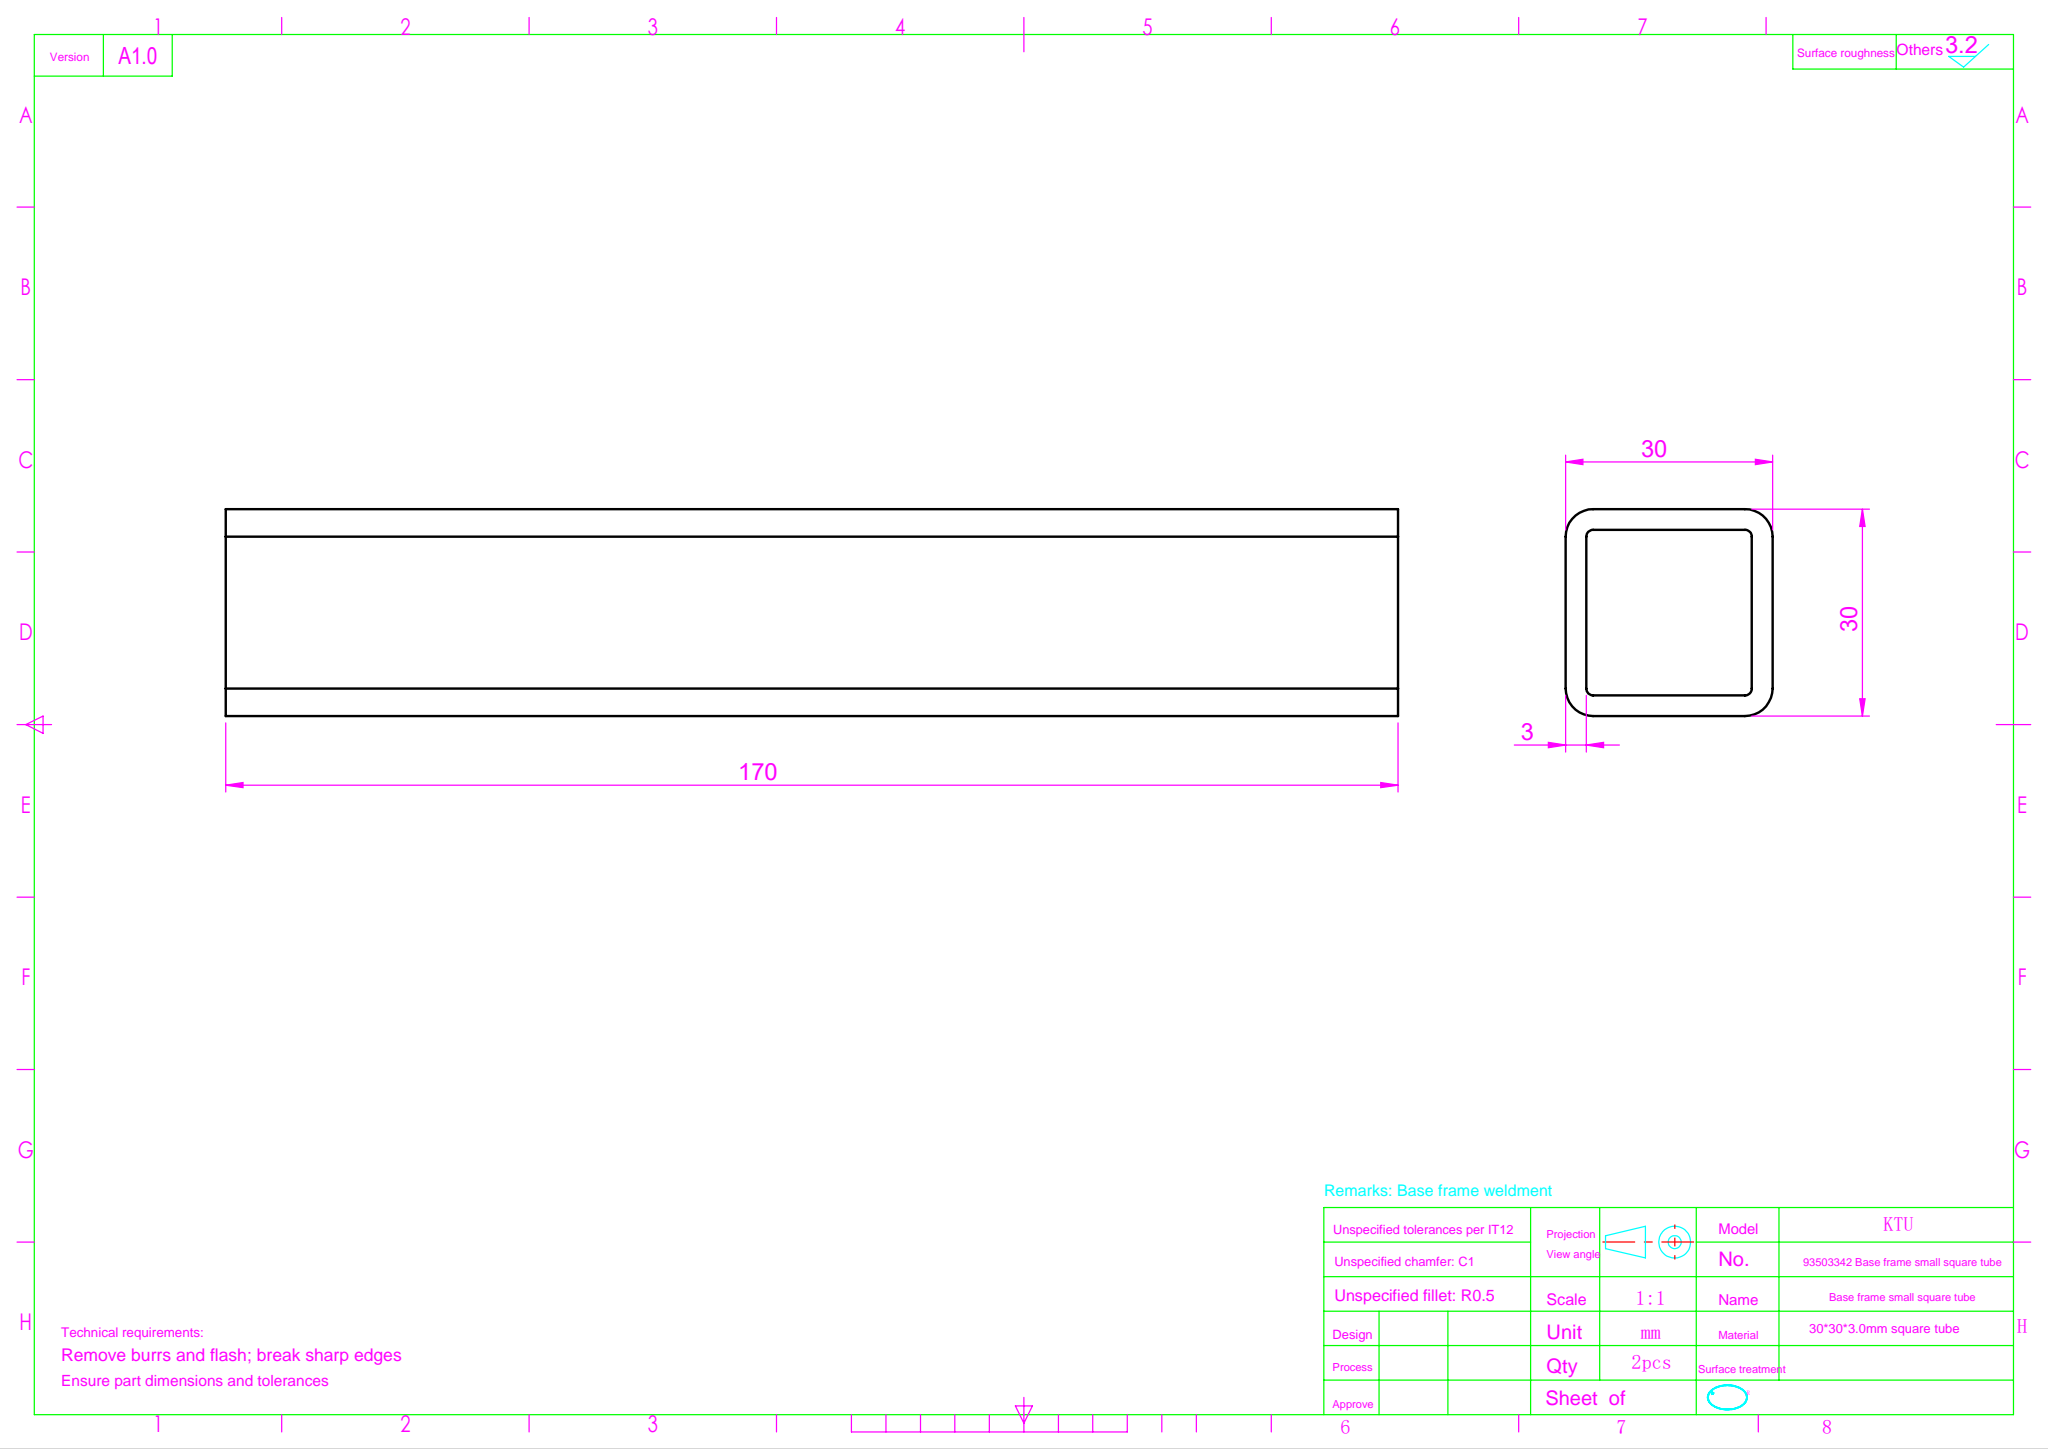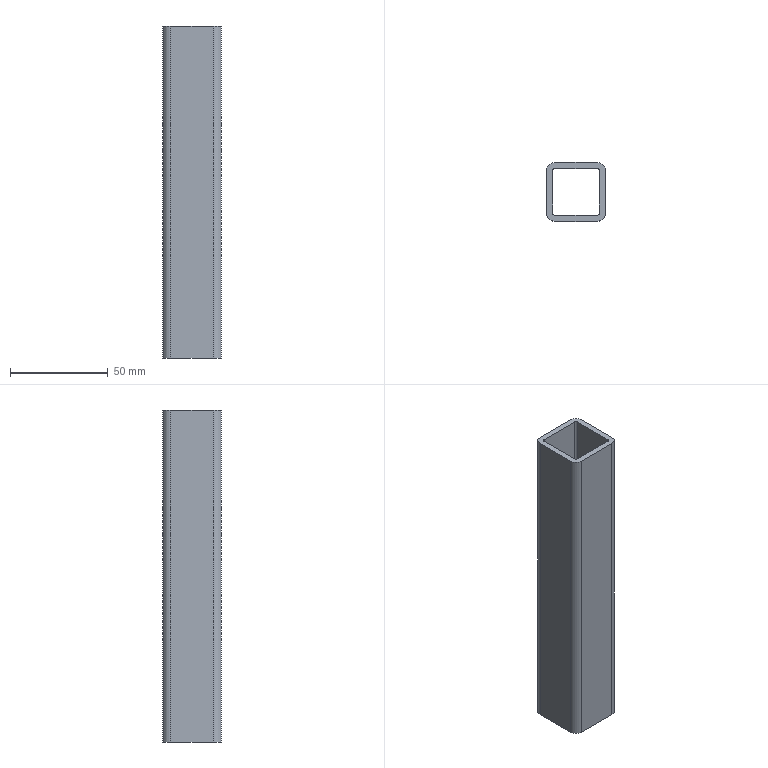Part | SolidWorks | features ExtruThin 1 | 1 solid | 18 faces | box 30 x 30 x 170 mm | volume 52891 mm3 | plane 10 | cylinder 8 | commonest cylinder face diameters 2 x4 8 x4
STEP:
#1=CARTESIAN_POINT('',(15.,11.,85.));
#2=VERTEX_POINT('',#1);
#3=CARTESIAN_POINT('',(11.,15.,85.));
#4=VERTEX_POINT('',#3);
#5=CARTESIAN_POINT('',(11.,11.,85.));
#6=DIRECTION('',(0.,0.,1.));
#7=DIRECTION('',(-1.,0.,0.));
#8=AXIS2_PLACEMENT_3D('',#5,#6,#7);
#9=CIRCLE('',#8,4.);
#10=EDGE_CURVE('',#2,#4,#9,.T.);
#11=ORIENTED_EDGE('',*,*,#10,.T.);
#12=CARTESIAN_POINT('',(-11.,15.,85.));
#13=VERTEX_POINT('',#12);
#14=CARTESIAN_POINT('',(-11.,15.,85.));
#15=DIRECTION('',(-1.,0.,0.));
#16=VECTOR('',#15,1000.);
#17=LINE('',#14,#16);
#18=EDGE_CURVE('',#4,#13,#17,.T.);
#19=ORIENTED_EDGE('',*,*,#18,.T.);
#20=CARTESIAN_POINT('',(-15.,11.,85.));
#21=VERTEX_POINT('',#20);
#22=CARTESIAN_POINT('',(-11.,11.,85.));
#23=DIRECTION('',(0.,0.,1.));
#24=DIRECTION('',(1.,0.,0.));
#25=AXIS2_PLACEMENT_3D('',#22,#23,#24);
#26=CIRCLE('',#25,4.);
#27=EDGE_CURVE('',#13,#21,#26,.T.);
#28=ORIENTED_EDGE('',*,*,#27,.T.);
#29=CARTESIAN_POINT('',(-15.,-11.,85.));
#30=VERTEX_POINT('',#29);
#31=CARTESIAN_POINT('',(-15.,11.,85.));
#32=DIRECTION('',(0.,-1.,0.));
#33=VECTOR('',#32,1000.);
#34=LINE('',#31,#33);
#35=EDGE_CURVE('',#21,#30,#34,.T.);
#36=ORIENTED_EDGE('',*,*,#35,.T.);
#37=CARTESIAN_POINT('',(-11.,-15.,85.));
#38=VERTEX_POINT('',#37);
#39=CARTESIAN_POINT('',(-11.,-11.,85.));
#40=DIRECTION('',(0.,0.,1.));
#41=DIRECTION('',(1.,0.,0.));
#42=AXIS2_PLACEMENT_3D('',#39,#40,#41);
#43=CIRCLE('',#42,4.);
#44=EDGE_CURVE('',#30,#38,#43,.T.);
#45=ORIENTED_EDGE('',*,*,#44,.T.);
#46=CARTESIAN_POINT('',(11.,-15.,85.));
#47=VERTEX_POINT('',#46);
#48=CARTESIAN_POINT('',(-11.,-15.,85.));
#49=DIRECTION('',(1.,0.,0.));
#50=VECTOR('',#49,1000.);
#51=LINE('',#48,#50);
#52=EDGE_CURVE('',#38,#47,#51,.T.);
#53=ORIENTED_EDGE('',*,*,#52,.T.);
#54=CARTESIAN_POINT('',(15.,-11.,85.));
#55=VERTEX_POINT('',#54);
#56=CARTESIAN_POINT('',(11.,-11.,85.));
#57=DIRECTION('',(0.,0.,1.));
#58=DIRECTION('',(1.,0.,0.));
#59=AXIS2_PLACEMENT_3D('',#56,#57,#58);
#60=CIRCLE('',#59,4.);
#61=EDGE_CURVE('',#47,#55,#60,.T.);
#62=ORIENTED_EDGE('',*,*,#61,.T.);
#63=CARTESIAN_POINT('',(15.,11.,85.));
#64=DIRECTION('',(0.,1.,0.));
#65=VECTOR('',#64,1000.);
#66=LINE('',#63,#65);
#67=EDGE_CURVE('',#55,#2,#66,.T.);
#68=ORIENTED_EDGE('',*,*,#67,.T.);
#69=EDGE_LOOP('',(#11,#19,#28,#36,#45,#53,#62,#68));
#70=FACE_OUTER_BOUND('',#69,.T.);
#71=CARTESIAN_POINT('',(11.,12.,85.));
#72=VERTEX_POINT('',#71);
#73=CARTESIAN_POINT('',(-11.,12.,85.));
#74=VERTEX_POINT('',#73);
#75=CARTESIAN_POINT('',(11.,12.,85.));
#76=DIRECTION('',(-1.,0.,0.));
#77=VECTOR('',#76,1000.);
#78=LINE('',#75,#77);
#79=EDGE_CURVE('',#72,#74,#78,.T.);
#80=ORIENTED_EDGE('',*,*,#79,.F.);
#81=CARTESIAN_POINT('',(12.,11.,85.));
#82=VERTEX_POINT('',#81);
#83=CARTESIAN_POINT('',(11.,11.,85.));
#84=DIRECTION('',(0.,0.,1.));
#85=DIRECTION('',(-1.,0.,0.));
#86=AXIS2_PLACEMENT_3D('',#83,#84,#85);
#87=CIRCLE('',#86,1.);
#88=EDGE_CURVE('',#82,#72,#87,.T.);
#89=ORIENTED_EDGE('',*,*,#88,.F.);
#90=CARTESIAN_POINT('',(12.,-11.,85.));
#91=VERTEX_POINT('',#90);
#92=CARTESIAN_POINT('',(12.,11.,85.));
#93=DIRECTION('',(0.,1.,0.));
#94=VECTOR('',#93,1000.);
#95=LINE('',#92,#94);
#96=EDGE_CURVE('',#91,#82,#95,.T.);
#97=ORIENTED_EDGE('',*,*,#96,.F.);
#98=CARTESIAN_POINT('',(11.,-12.,85.));
#99=VERTEX_POINT('',#98);
#100=CARTESIAN_POINT('',(11.,-11.,85.));
#101=DIRECTION('',(0.,0.,1.));
#102=DIRECTION('',(-1.,0.,0.));
#103=AXIS2_PLACEMENT_3D('',#100,#101,#102);
#104=CIRCLE('',#103,1.);
#105=EDGE_CURVE('',#99,#91,#104,.T.);
#106=ORIENTED_EDGE('',*,*,#105,.F.);
#107=CARTESIAN_POINT('',(-11.,-12.,85.));
#108=VERTEX_POINT('',#107);
#109=CARTESIAN_POINT('',(11.,-12.,85.));
#110=DIRECTION('',(1.,0.,0.));
#111=VECTOR('',#110,1000.);
#112=LINE('',#109,#111);
#113=EDGE_CURVE('',#108,#99,#112,.T.);
#114=ORIENTED_EDGE('',*,*,#113,.F.);
#115=CARTESIAN_POINT('',(-12.,-11.,85.));
#116=VERTEX_POINT('',#115);
#117=CARTESIAN_POINT('',(-11.,-11.,85.));
#118=DIRECTION('',(0.,0.,1.));
#119=DIRECTION('',(-1.,0.,0.));
#120=AXIS2_PLACEMENT_3D('',#117,#118,#119);
#121=CIRCLE('',#120,1.);
#122=EDGE_CURVE('',#116,#108,#121,.T.);
#123=ORIENTED_EDGE('',*,*,#122,.F.);
#124=CARTESIAN_POINT('',(-12.,11.,85.));
#125=VERTEX_POINT('',#124);
#126=CARTESIAN_POINT('',(-12.,11.,85.));
#127=DIRECTION('',(0.,-1.,0.));
#128=VECTOR('',#127,1000.);
#129=LINE('',#126,#128);
#130=EDGE_CURVE('',#125,#116,#129,.T.);
#131=ORIENTED_EDGE('',*,*,#130,.F.);
#132=CARTESIAN_POINT('',(-11.,11.,85.));
#133=DIRECTION('',(0.,0.,1.));
#134=DIRECTION('',(-1.,0.,0.));
#135=AXIS2_PLACEMENT_3D('',#132,#133,#134);
#136=CIRCLE('',#135,1.);
#137=EDGE_CURVE('',#74,#125,#136,.T.);
#138=ORIENTED_EDGE('',*,*,#137,.F.);
#139=EDGE_LOOP('',(#80,#89,#97,#106,#114,#123,#131,#138));
#140=FACE_BOUND('',#139,.T.);
#141=CARTESIAN_POINT('',(11.,11.,85.));
#142=DIRECTION('',(0.,0.,1.));
#143=DIRECTION('',(1.,0.,0.));
#144=AXIS2_PLACEMENT_3D('',#141,#142,#143);
#145=PLANE('',#144);
#146=ADVANCED_FACE('',(#70,#140),#145,.T.);
#147=CARTESIAN_POINT('',(15.,11.,-85.));
#148=VERTEX_POINT('',#147);
#149=CARTESIAN_POINT('',(11.,15.,-85.));
#150=VERTEX_POINT('',#149);
#151=CARTESIAN_POINT('',(11.,11.,-85.));
#152=DIRECTION('',(0.,0.,1.));
#153=DIRECTION('',(-1.,0.,0.));
#154=AXIS2_PLACEMENT_3D('',#151,#152,#153);
#155=CIRCLE('',#154,4.);
#156=EDGE_CURVE('',#148,#150,#155,.T.);
#157=ORIENTED_EDGE('',*,*,#156,.F.);
#158=CARTESIAN_POINT('',(15.,-11.,-85.));
#159=VERTEX_POINT('',#158);
#160=CARTESIAN_POINT('',(15.,11.,-85.));
#161=DIRECTION('',(0.,1.,0.));
#162=VECTOR('',#161,1000.);
#163=LINE('',#160,#162);
#164=EDGE_CURVE('',#159,#148,#163,.T.);
#165=ORIENTED_EDGE('',*,*,#164,.F.);
#166=CARTESIAN_POINT('',(11.,-15.,-85.));
#167=VERTEX_POINT('',#166);
#168=CARTESIAN_POINT('',(11.,-11.,-85.));
#169=DIRECTION('',(0.,0.,1.));
#170=DIRECTION('',(1.,0.,0.));
#171=AXIS2_PLACEMENT_3D('',#168,#169,#170);
#172=CIRCLE('',#171,4.);
#173=EDGE_CURVE('',#167,#159,#172,.T.);
#174=ORIENTED_EDGE('',*,*,#173,.F.);
#175=CARTESIAN_POINT('',(-11.,-15.,-85.));
#176=VERTEX_POINT('',#175);
#177=CARTESIAN_POINT('',(-11.,-15.,-85.));
#178=DIRECTION('',(1.,0.,0.));
#179=VECTOR('',#178,1000.);
#180=LINE('',#177,#179);
#181=EDGE_CURVE('',#176,#167,#180,.T.);
#182=ORIENTED_EDGE('',*,*,#181,.F.);
#183=CARTESIAN_POINT('',(-15.,-11.,-85.));
#184=VERTEX_POINT('',#183);
#185=CARTESIAN_POINT('',(-11.,-11.,-85.));
#186=DIRECTION('',(0.,0.,1.));
#187=DIRECTION('',(1.,0.,0.));
#188=AXIS2_PLACEMENT_3D('',#185,#186,#187);
#189=CIRCLE('',#188,4.);
#190=EDGE_CURVE('',#184,#176,#189,.T.);
#191=ORIENTED_EDGE('',*,*,#190,.F.);
#192=CARTESIAN_POINT('',(-15.,11.,-85.));
#193=VERTEX_POINT('',#192);
#194=CARTESIAN_POINT('',(-15.,11.,-85.));
#195=DIRECTION('',(0.,-1.,0.));
#196=VECTOR('',#195,1000.);
#197=LINE('',#194,#196);
#198=EDGE_CURVE('',#193,#184,#197,.T.);
#199=ORIENTED_EDGE('',*,*,#198,.F.);
#200=CARTESIAN_POINT('',(-11.,15.,-85.));
#201=VERTEX_POINT('',#200);
#202=CARTESIAN_POINT('',(-11.,11.,-85.));
#203=DIRECTION('',(0.,0.,1.));
#204=DIRECTION('',(1.,0.,0.));
#205=AXIS2_PLACEMENT_3D('',#202,#203,#204);
#206=CIRCLE('',#205,4.);
#207=EDGE_CURVE('',#201,#193,#206,.T.);
#208=ORIENTED_EDGE('',*,*,#207,.F.);
#209=CARTESIAN_POINT('',(-11.,15.,-85.));
#210=DIRECTION('',(-1.,0.,0.));
#211=VECTOR('',#210,1000.);
#212=LINE('',#209,#211);
#213=EDGE_CURVE('',#150,#201,#212,.T.);
#214=ORIENTED_EDGE('',*,*,#213,.F.);
#215=EDGE_LOOP('',(#157,#165,#174,#182,#191,#199,#208,#214));
#216=FACE_OUTER_BOUND('',#215,.T.);
#217=CARTESIAN_POINT('',(12.,11.,-85.));
#218=VERTEX_POINT('',#217);
#219=CARTESIAN_POINT('',(11.,12.,-85.));
#220=VERTEX_POINT('',#219);
#221=CARTESIAN_POINT('',(11.,11.,-85.));
#222=DIRECTION('',(0.,0.,1.));
#223=DIRECTION('',(-1.,0.,0.));
#224=AXIS2_PLACEMENT_3D('',#221,#222,#223);
#225=CIRCLE('',#224,1.);
#226=EDGE_CURVE('',#218,#220,#225,.T.);
#227=ORIENTED_EDGE('',*,*,#226,.T.);
#228=CARTESIAN_POINT('',(-11.,12.,-85.));
#229=VERTEX_POINT('',#228);
#230=CARTESIAN_POINT('',(11.,12.,-85.));
#231=DIRECTION('',(-1.,0.,0.));
#232=VECTOR('',#231,1000.);
#233=LINE('',#230,#232);
#234=EDGE_CURVE('',#220,#229,#233,.T.);
#235=ORIENTED_EDGE('',*,*,#234,.T.);
#236=CARTESIAN_POINT('',(-12.,11.,-85.));
#237=VERTEX_POINT('',#236);
#238=CARTESIAN_POINT('',(-11.,11.,-85.));
#239=DIRECTION('',(0.,0.,1.));
#240=DIRECTION('',(-1.,0.,0.));
#241=AXIS2_PLACEMENT_3D('',#238,#239,#240);
#242=CIRCLE('',#241,1.);
#243=EDGE_CURVE('',#229,#237,#242,.T.);
#244=ORIENTED_EDGE('',*,*,#243,.T.);
#245=CARTESIAN_POINT('',(-12.,-11.,-85.));
#246=VERTEX_POINT('',#245);
#247=CARTESIAN_POINT('',(-12.,11.,-85.));
#248=DIRECTION('',(0.,-1.,0.));
#249=VECTOR('',#248,1000.);
#250=LINE('',#247,#249);
#251=EDGE_CURVE('',#237,#246,#250,.T.);
#252=ORIENTED_EDGE('',*,*,#251,.T.);
#253=CARTESIAN_POINT('',(-11.,-12.,-85.));
#254=VERTEX_POINT('',#253);
#255=CARTESIAN_POINT('',(-11.,-11.,-85.));
#256=DIRECTION('',(0.,0.,1.));
#257=DIRECTION('',(-1.,0.,0.));
#258=AXIS2_PLACEMENT_3D('',#255,#256,#257);
#259=CIRCLE('',#258,1.);
#260=EDGE_CURVE('',#246,#254,#259,.T.);
#261=ORIENTED_EDGE('',*,*,#260,.T.);
#262=CARTESIAN_POINT('',(11.,-12.,-85.));
#263=VERTEX_POINT('',#262);
#264=CARTESIAN_POINT('',(11.,-12.,-85.));
#265=DIRECTION('',(1.,0.,0.));
#266=VECTOR('',#265,1000.);
#267=LINE('',#264,#266);
#268=EDGE_CURVE('',#254,#263,#267,.T.);
#269=ORIENTED_EDGE('',*,*,#268,.T.);
#270=CARTESIAN_POINT('',(12.,-11.,-85.));
#271=VERTEX_POINT('',#270);
#272=CARTESIAN_POINT('',(11.,-11.,-85.));
#273=DIRECTION('',(0.,0.,1.));
#274=DIRECTION('',(-1.,0.,0.));
#275=AXIS2_PLACEMENT_3D('',#272,#273,#274);
#276=CIRCLE('',#275,1.);
#277=EDGE_CURVE('',#263,#271,#276,.T.);
#278=ORIENTED_EDGE('',*,*,#277,.T.);
#279=CARTESIAN_POINT('',(12.,11.,-85.));
#280=DIRECTION('',(0.,1.,0.));
#281=VECTOR('',#280,1000.);
#282=LINE('',#279,#281);
#283=EDGE_CURVE('',#271,#218,#282,.T.);
#284=ORIENTED_EDGE('',*,*,#283,.T.);
#285=EDGE_LOOP('',(#227,#235,#244,#252,#261,#269,#278,#284));
#286=FACE_BOUND('',#285,.T.);
#287=CARTESIAN_POINT('',(11.,11.,-85.));
#288=DIRECTION('',(0.,0.,1.));
#289=DIRECTION('',(1.,0.,0.));
#290=AXIS2_PLACEMENT_3D('',#287,#288,#289);
#291=PLANE('',#290);
#292=ADVANCED_FACE('',(#216,#286),#291,.F.);
#293=ORIENTED_EDGE('',*,*,#156,.T.);
#294=CARTESIAN_POINT('',(11.,15.,85.));
#295=DIRECTION('',(0.,0.,-1.));
#296=VECTOR('',#295,1000.);
#297=LINE('',#294,#296);
#298=EDGE_CURVE('',#4,#150,#297,.T.);
#299=ORIENTED_EDGE('',*,*,#298,.F.);
#300=ORIENTED_EDGE('',*,*,#10,.F.);
#301=CARTESIAN_POINT('',(15.,11.,85.));
#302=DIRECTION('',(0.,0.,-1.));
#303=VECTOR('',#302,1000.);
#304=LINE('',#301,#303);
#305=EDGE_CURVE('',#2,#148,#304,.T.);
#306=ORIENTED_EDGE('',*,*,#305,.T.);
#307=EDGE_LOOP('',(#293,#299,#300,#306));
#308=FACE_OUTER_BOUND('',#307,.T.);
#309=CARTESIAN_POINT('',(11.,11.,85.));
#310=DIRECTION('',(0.,0.,-1.));
#311=DIRECTION('',(-1.,0.,0.));
#312=AXIS2_PLACEMENT_3D('',#309,#310,#311);
#313=CYLINDRICAL_SURFACE('',#312,4.);
#314=ADVANCED_FACE('',(#308),#313,.T.);
#315=ORIENTED_EDGE('',*,*,#213,.T.);
#316=CARTESIAN_POINT('',(-11.,15.,85.));
#317=DIRECTION('',(0.,0.,-1.));
#318=VECTOR('',#317,1000.);
#319=LINE('',#316,#318);
#320=EDGE_CURVE('',#13,#201,#319,.T.);
#321=ORIENTED_EDGE('',*,*,#320,.F.);
#322=ORIENTED_EDGE('',*,*,#18,.F.);
#323=ORIENTED_EDGE('',*,*,#298,.T.);
#324=EDGE_LOOP('',(#315,#321,#322,#323));
#325=FACE_OUTER_BOUND('',#324,.T.);
#326=CARTESIAN_POINT('',(-11.,15.,85.));
#327=DIRECTION('',(0.,-1.,0.));
#328=DIRECTION('',(0.,0.,-1.));
#329=AXIS2_PLACEMENT_3D('',#326,#327,#328);
#330=PLANE('',#329);
#331=ADVANCED_FACE('',(#325),#330,.F.);
#332=ORIENTED_EDGE('',*,*,#207,.T.);
#333=CARTESIAN_POINT('',(-15.,11.,85.));
#334=DIRECTION('',(0.,0.,-1.));
#335=VECTOR('',#334,1000.);
#336=LINE('',#333,#335);
#337=EDGE_CURVE('',#21,#193,#336,.T.);
#338=ORIENTED_EDGE('',*,*,#337,.F.);
#339=ORIENTED_EDGE('',*,*,#27,.F.);
#340=ORIENTED_EDGE('',*,*,#320,.T.);
#341=EDGE_LOOP('',(#332,#338,#339,#340));
#342=FACE_OUTER_BOUND('',#341,.T.);
#343=CARTESIAN_POINT('',(-11.,11.,85.));
#344=DIRECTION('',(0.,0.,-1.));
#345=DIRECTION('',(-1.,0.,0.));
#346=AXIS2_PLACEMENT_3D('',#343,#344,#345);
#347=CYLINDRICAL_SURFACE('',#346,4.);
#348=ADVANCED_FACE('',(#342),#347,.T.);
#349=ORIENTED_EDGE('',*,*,#198,.T.);
#350=CARTESIAN_POINT('',(-15.,-11.,85.));
#351=DIRECTION('',(0.,0.,-1.));
#352=VECTOR('',#351,1000.);
#353=LINE('',#350,#352);
#354=EDGE_CURVE('',#30,#184,#353,.T.);
#355=ORIENTED_EDGE('',*,*,#354,.F.);
#356=ORIENTED_EDGE('',*,*,#35,.F.);
#357=ORIENTED_EDGE('',*,*,#337,.T.);
#358=EDGE_LOOP('',(#349,#355,#356,#357));
#359=FACE_OUTER_BOUND('',#358,.T.);
#360=CARTESIAN_POINT('',(-15.,11.,85.));
#361=DIRECTION('',(1.,0.,0.));
#362=DIRECTION('',(0.,1.,0.));
#363=AXIS2_PLACEMENT_3D('',#360,#361,#362);
#364=PLANE('',#363);
#365=ADVANCED_FACE('',(#359),#364,.F.);
#366=ORIENTED_EDGE('',*,*,#190,.T.);
#367=CARTESIAN_POINT('',(-11.,-15.,85.));
#368=DIRECTION('',(0.,0.,-1.));
#369=VECTOR('',#368,1000.);
#370=LINE('',#367,#369);
#371=EDGE_CURVE('',#38,#176,#370,.T.);
#372=ORIENTED_EDGE('',*,*,#371,.F.);
#373=ORIENTED_EDGE('',*,*,#44,.F.);
#374=ORIENTED_EDGE('',*,*,#354,.T.);
#375=EDGE_LOOP('',(#366,#372,#373,#374));
#376=FACE_OUTER_BOUND('',#375,.T.);
#377=CARTESIAN_POINT('',(-11.,-11.,85.));
#378=DIRECTION('',(0.,0.,-1.));
#379=DIRECTION('',(-1.,0.,0.));
#380=AXIS2_PLACEMENT_3D('',#377,#378,#379);
#381=CYLINDRICAL_SURFACE('',#380,4.);
#382=ADVANCED_FACE('',(#376),#381,.T.);
#383=ORIENTED_EDGE('',*,*,#181,.T.);
#384=CARTESIAN_POINT('',(11.,-15.,85.));
#385=DIRECTION('',(0.,0.,-1.));
#386=VECTOR('',#385,1000.);
#387=LINE('',#384,#386);
#388=EDGE_CURVE('',#47,#167,#387,.T.);
#389=ORIENTED_EDGE('',*,*,#388,.F.);
#390=ORIENTED_EDGE('',*,*,#52,.F.);
#391=ORIENTED_EDGE('',*,*,#371,.T.);
#392=EDGE_LOOP('',(#383,#389,#390,#391));
#393=FACE_OUTER_BOUND('',#392,.T.);
#394=CARTESIAN_POINT('',(-11.,-15.,85.));
#395=DIRECTION('',(0.,1.,0.));
#396=DIRECTION('',(0.,0.,1.));
#397=AXIS2_PLACEMENT_3D('',#394,#395,#396);
#398=PLANE('',#397);
#399=ADVANCED_FACE('',(#393),#398,.F.);
#400=ORIENTED_EDGE('',*,*,#173,.T.);
#401=CARTESIAN_POINT('',(15.,-11.,85.));
#402=DIRECTION('',(0.,0.,-1.));
#403=VECTOR('',#402,1000.);
#404=LINE('',#401,#403);
#405=EDGE_CURVE('',#55,#159,#404,.T.);
#406=ORIENTED_EDGE('',*,*,#405,.F.);
#407=ORIENTED_EDGE('',*,*,#61,.F.);
#408=ORIENTED_EDGE('',*,*,#388,.T.);
#409=EDGE_LOOP('',(#400,#406,#407,#408));
#410=FACE_OUTER_BOUND('',#409,.T.);
#411=CARTESIAN_POINT('',(11.,-11.,85.));
#412=DIRECTION('',(0.,0.,-1.));
#413=DIRECTION('',(-1.,0.,0.));
#414=AXIS2_PLACEMENT_3D('',#411,#412,#413);
#415=CYLINDRICAL_SURFACE('',#414,4.);
#416=ADVANCED_FACE('',(#410),#415,.T.);
#417=ORIENTED_EDGE('',*,*,#164,.T.);
#418=ORIENTED_EDGE('',*,*,#305,.F.);
#419=ORIENTED_EDGE('',*,*,#67,.F.);
#420=ORIENTED_EDGE('',*,*,#405,.T.);
#421=EDGE_LOOP('',(#417,#418,#419,#420));
#422=FACE_OUTER_BOUND('',#421,.T.);
#423=CARTESIAN_POINT('',(15.,11.,85.));
#424=DIRECTION('',(-1.,0.,0.));
#425=DIRECTION('',(0.,-1.,0.));
#426=AXIS2_PLACEMENT_3D('',#423,#424,#425);
#427=PLANE('',#426);
#428=ADVANCED_FACE('',(#422),#427,.F.);
#429=ORIENTED_EDGE('',*,*,#226,.F.);
#430=CARTESIAN_POINT('',(12.,11.,85.));
#431=DIRECTION('',(0.,0.,-1.));
#432=VECTOR('',#431,1000.);
#433=LINE('',#430,#432);
#434=EDGE_CURVE('',#82,#218,#433,.T.);
#435=ORIENTED_EDGE('',*,*,#434,.F.);
#436=ORIENTED_EDGE('',*,*,#88,.T.);
#437=CARTESIAN_POINT('',(11.,12.,85.));
#438=DIRECTION('',(0.,0.,-1.));
#439=VECTOR('',#438,1000.);
#440=LINE('',#437,#439);
#441=EDGE_CURVE('',#72,#220,#440,.T.);
#442=ORIENTED_EDGE('',*,*,#441,.T.);
#443=EDGE_LOOP('',(#429,#435,#436,#442));
#444=FACE_OUTER_BOUND('',#443,.T.);
#445=CARTESIAN_POINT('',(11.,11.,85.));
#446=DIRECTION('',(0.,0.,-1.));
#447=DIRECTION('',(-1.,0.,0.));
#448=AXIS2_PLACEMENT_3D('',#445,#446,#447);
#449=CYLINDRICAL_SURFACE('',#448,1.);
#450=ADVANCED_FACE('',(#444),#449,.F.);
#451=ORIENTED_EDGE('',*,*,#234,.F.);
#452=ORIENTED_EDGE('',*,*,#441,.F.);
#453=ORIENTED_EDGE('',*,*,#79,.T.);
#454=CARTESIAN_POINT('',(-11.,12.,85.));
#455=DIRECTION('',(0.,0.,-1.));
#456=VECTOR('',#455,1000.);
#457=LINE('',#454,#456);
#458=EDGE_CURVE('',#74,#229,#457,.T.);
#459=ORIENTED_EDGE('',*,*,#458,.T.);
#460=EDGE_LOOP('',(#451,#452,#453,#459));
#461=FACE_OUTER_BOUND('',#460,.T.);
#462=CARTESIAN_POINT('',(11.,12.,85.));
#463=DIRECTION('',(0.,-1.,0.));
#464=DIRECTION('',(0.,0.,-1.));
#465=AXIS2_PLACEMENT_3D('',#462,#463,#464);
#466=PLANE('',#465);
#467=ADVANCED_FACE('',(#461),#466,.T.);
#468=ORIENTED_EDGE('',*,*,#243,.F.);
#469=ORIENTED_EDGE('',*,*,#458,.F.);
#470=ORIENTED_EDGE('',*,*,#137,.T.);
#471=CARTESIAN_POINT('',(-12.,11.,85.));
#472=DIRECTION('',(0.,0.,-1.));
#473=VECTOR('',#472,1000.);
#474=LINE('',#471,#473);
#475=EDGE_CURVE('',#125,#237,#474,.T.);
#476=ORIENTED_EDGE('',*,*,#475,.T.);
#477=EDGE_LOOP('',(#468,#469,#470,#476));
#478=FACE_OUTER_BOUND('',#477,.T.);
#479=CARTESIAN_POINT('',(-11.,11.,85.));
#480=DIRECTION('',(0.,0.,-1.));
#481=DIRECTION('',(-1.,0.,0.));
#482=AXIS2_PLACEMENT_3D('',#479,#480,#481);
#483=CYLINDRICAL_SURFACE('',#482,1.);
#484=ADVANCED_FACE('',(#478),#483,.F.);
#485=ORIENTED_EDGE('',*,*,#251,.F.);
#486=ORIENTED_EDGE('',*,*,#475,.F.);
#487=ORIENTED_EDGE('',*,*,#130,.T.);
#488=CARTESIAN_POINT('',(-12.,-11.,85.));
#489=DIRECTION('',(0.,0.,-1.));
#490=VECTOR('',#489,1000.);
#491=LINE('',#488,#490);
#492=EDGE_CURVE('',#116,#246,#491,.T.);
#493=ORIENTED_EDGE('',*,*,#492,.T.);
#494=EDGE_LOOP('',(#485,#486,#487,#493));
#495=FACE_OUTER_BOUND('',#494,.T.);
#496=CARTESIAN_POINT('',(-12.,11.,85.));
#497=DIRECTION('',(1.,0.,0.));
#498=DIRECTION('',(0.,1.,0.));
#499=AXIS2_PLACEMENT_3D('',#496,#497,#498);
#500=PLANE('',#499);
#501=ADVANCED_FACE('',(#495),#500,.T.);
#502=ORIENTED_EDGE('',*,*,#260,.F.);
#503=ORIENTED_EDGE('',*,*,#492,.F.);
#504=ORIENTED_EDGE('',*,*,#122,.T.);
#505=CARTESIAN_POINT('',(-11.,-12.,85.));
#506=DIRECTION('',(0.,0.,-1.));
#507=VECTOR('',#506,1000.);
#508=LINE('',#505,#507);
#509=EDGE_CURVE('',#108,#254,#508,.T.);
#510=ORIENTED_EDGE('',*,*,#509,.T.);
#511=EDGE_LOOP('',(#502,#503,#504,#510));
#512=FACE_OUTER_BOUND('',#511,.T.);
#513=CARTESIAN_POINT('',(-11.,-11.,85.));
#514=DIRECTION('',(0.,0.,-1.));
#515=DIRECTION('',(-1.,0.,0.));
#516=AXIS2_PLACEMENT_3D('',#513,#514,#515);
#517=CYLINDRICAL_SURFACE('',#516,1.);
#518=ADVANCED_FACE('',(#512),#517,.F.);
#519=ORIENTED_EDGE('',*,*,#268,.F.);
#520=ORIENTED_EDGE('',*,*,#509,.F.);
#521=ORIENTED_EDGE('',*,*,#113,.T.);
#522=CARTESIAN_POINT('',(11.,-12.,85.));
#523=DIRECTION('',(0.,0.,-1.));
#524=VECTOR('',#523,1000.);
#525=LINE('',#522,#524);
#526=EDGE_CURVE('',#99,#263,#525,.T.);
#527=ORIENTED_EDGE('',*,*,#526,.T.);
#528=EDGE_LOOP('',(#519,#520,#521,#527));
#529=FACE_OUTER_BOUND('',#528,.T.);
#530=CARTESIAN_POINT('',(11.,-12.,85.));
#531=DIRECTION('',(0.,1.,0.));
#532=DIRECTION('',(0.,0.,1.));
#533=AXIS2_PLACEMENT_3D('',#530,#531,#532);
#534=PLANE('',#533);
#535=ADVANCED_FACE('',(#529),#534,.T.);
#536=ORIENTED_EDGE('',*,*,#277,.F.);
#537=ORIENTED_EDGE('',*,*,#526,.F.);
#538=ORIENTED_EDGE('',*,*,#105,.T.);
#539=CARTESIAN_POINT('',(12.,-11.,85.));
#540=DIRECTION('',(0.,0.,-1.));
#541=VECTOR('',#540,1000.);
#542=LINE('',#539,#541);
#543=EDGE_CURVE('',#91,#271,#542,.T.);
#544=ORIENTED_EDGE('',*,*,#543,.T.);
#545=EDGE_LOOP('',(#536,#537,#538,#544));
#546=FACE_OUTER_BOUND('',#545,.T.);
#547=CARTESIAN_POINT('',(11.,-11.,85.));
#548=DIRECTION('',(0.,0.,-1.));
#549=DIRECTION('',(-1.,0.,0.));
#550=AXIS2_PLACEMENT_3D('',#547,#548,#549);
#551=CYLINDRICAL_SURFACE('',#550,1.);
#552=ADVANCED_FACE('',(#546),#551,.F.);
#553=ORIENTED_EDGE('',*,*,#283,.F.);
#554=ORIENTED_EDGE('',*,*,#543,.F.);
#555=ORIENTED_EDGE('',*,*,#96,.T.);
#556=ORIENTED_EDGE('',*,*,#434,.T.);
#557=EDGE_LOOP('',(#553,#554,#555,#556));
#558=FACE_OUTER_BOUND('',#557,.T.);
#559=CARTESIAN_POINT('',(12.,11.,85.));
#560=DIRECTION('',(-1.,0.,0.));
#561=DIRECTION('',(0.,-1.,0.));
#562=AXIS2_PLACEMENT_3D('',#559,#560,#561);
#563=PLANE('',#562);
#564=ADVANCED_FACE('',(#558),#563,.T.);
#565=CLOSED_SHELL('',(#146,#292,#314,#331,#348,#365,#382,#399,#416,#428,#450,#467,#484,#501,#518,#535,#552,#564));
#566=MANIFOLD_SOLID_BREP('',#565);
#567=CARTESIAN_POINT('',(0.,0.,0.));
#568=DIRECTION('',(0.,0.,1.));
#569=DIRECTION('',(1.,0.,0.));
#570=AXIS2_PLACEMENT_3D('',#567,#568,#569);
#571=(LENGTH_UNIT()NAMED_UNIT(*)SI_UNIT(.MILLI.,.METRE.));
#572=UNCERTAINTY_MEASURE_WITH_UNIT(LENGTH_MEASURE(0.00001),#571,'','');
#573=(NAMED_UNIT(*)PLANE_ANGLE_UNIT()SI_UNIT($,.RADIAN.));
#574=(NAMED_UNIT(*)SI_UNIT($,.STERADIAN.)SOLID_ANGLE_UNIT());
#575=(GEOMETRIC_REPRESENTATION_CONTEXT(3)GLOBAL_UNCERTAINTY_ASSIGNED_CONTEXT((#572))GLOBAL_UNIT_ASSIGNED_CONTEXT((#571,#573,#574))REPRESENTATION_CONTEXT('',''));
#576=ADVANCED_BREP_SHAPE_REPRESENTATION('',(#566,#570),#575);